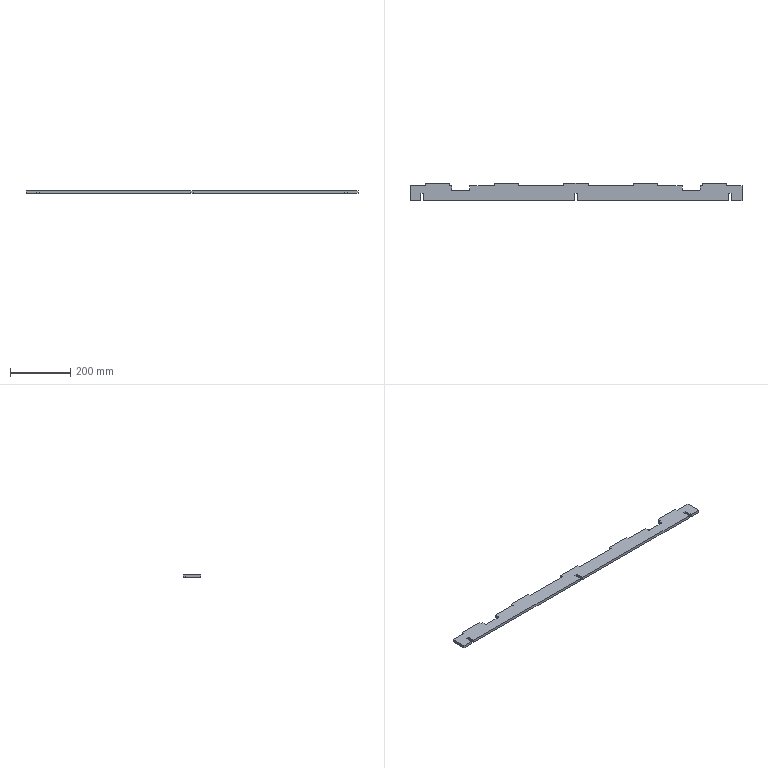Part | SolidWorks | features FlatPattern 1, SMBaseFlange 1, SheetMetal 1 | 1 solid | 50 faces | box 1100 x 58.5 x 9 mm | volume 503273 mm3 | plane 46 | cylinder 4 | commonest cylinder face diameters 6 x4